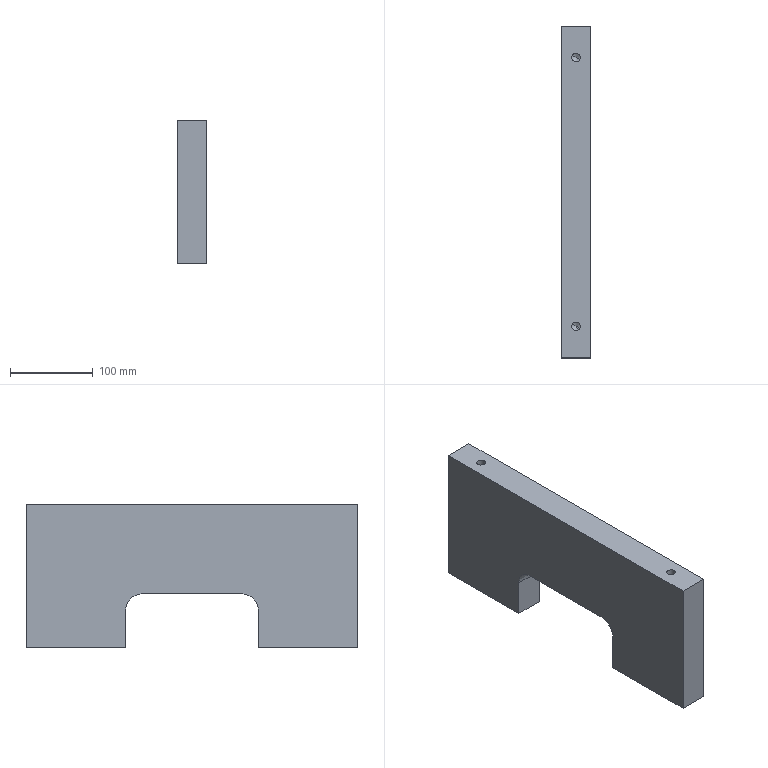Part | CATIA | 1 solid | 28 faces | box 35 x 400 x 173 mm | volume 2052248 mm3 | plane 10 | cylinder 10 | cone 8 | commonest cylinder face diameters 10.2 x8 40 x2
STEP:
#1=CARTESIAN_POINT('',(17.5,200.,-102.));
#2=VERTEX_POINT('',#1);
#3=CARTESIAN_POINT('',(17.5,200.,-275.));
#4=VERTEX_POINT('',#3);
#5=CARTESIAN_POINT('',(17.5,200.,-188.5));
#6=DIRECTION('',(0.,0.,-1.));
#7=VECTOR('',#6,1.);
#8=LINE('',#5,#7);
#9=EDGE_CURVE('',#2,#4,#8,.T.);
#10=ORIENTED_EDGE('',*,*,#9,.T.);
#11=CARTESIAN_POINT('',(-17.5,200.,-275.));
#12=VERTEX_POINT('',#11);
#13=CARTESIAN_POINT('',(0.,200.,-275.));
#14=DIRECTION('',(1.,0.,0.));
#15=VECTOR('',#14,1.);
#16=LINE('',#13,#15);
#17=EDGE_CURVE('',#4,#12,#16,.F.);
#18=ORIENTED_EDGE('',*,*,#17,.T.);
#19=CARTESIAN_POINT('',(-17.5,200.,-102.));
#20=VERTEX_POINT('',#19);
#21=CARTESIAN_POINT('',(-17.5,200.,-188.5));
#22=DIRECTION('',(0.,0.,-1.));
#23=VECTOR('',#22,1.);
#24=LINE('',#21,#23);
#25=EDGE_CURVE('',#20,#12,#24,.T.);
#26=ORIENTED_EDGE('',*,*,#25,.F.);
#27=CARTESIAN_POINT('',(0.,200.,-102.));
#28=DIRECTION('',(1.,0.,0.));
#29=VECTOR('',#28,1.);
#30=LINE('',#27,#29);
#31=EDGE_CURVE('',#20,#2,#30,.T.);
#32=ORIENTED_EDGE('',*,*,#31,.T.);
#33=EDGE_LOOP('',(#10,#18,#26,#32));
#34=FACE_OUTER_BOUND('',#33,.T.);
#35=CARTESIAN_POINT('',(-17.5,200.,0.));
#36=DIRECTION('',(0.,1.,0.));
#37=DIRECTION('',(1.,0.,0.));
#38=AXIS2_PLACEMENT_3D('',#35,#36,#37);
#39=PLANE('',#38);
#40=ADVANCED_FACE('',(#34),#39,.T.);
#41=CARTESIAN_POINT('',(-17.5,-200.,-102.));
#42=VERTEX_POINT('',#41);
#43=CARTESIAN_POINT('',(-17.5,-200.,-275.));
#44=VERTEX_POINT('',#43);
#45=CARTESIAN_POINT('',(-17.5,-200.,-188.5));
#46=DIRECTION('',(0.,0.,-1.));
#47=VECTOR('',#46,1.);
#48=LINE('',#45,#47);
#49=EDGE_CURVE('',#42,#44,#48,.T.);
#50=ORIENTED_EDGE('',*,*,#49,.T.);
#51=CARTESIAN_POINT('',(17.5,-200.,-275.));
#52=VERTEX_POINT('',#51);
#53=CARTESIAN_POINT('',(0.,-200.,-275.));
#54=DIRECTION('',(-1.,0.,0.));
#55=VECTOR('',#54,1.);
#56=LINE('',#53,#55);
#57=EDGE_CURVE('',#44,#52,#56,.F.);
#58=ORIENTED_EDGE('',*,*,#57,.T.);
#59=CARTESIAN_POINT('',(17.5,-200.,-102.));
#60=VERTEX_POINT('',#59);
#61=CARTESIAN_POINT('',(17.5,-200.,-188.5));
#62=DIRECTION('',(0.,0.,-1.));
#63=VECTOR('',#62,1.);
#64=LINE('',#61,#63);
#65=EDGE_CURVE('',#60,#52,#64,.T.);
#66=ORIENTED_EDGE('',*,*,#65,.F.);
#67=CARTESIAN_POINT('',(0.,-200.,-102.));
#68=DIRECTION('',(-1.,0.,0.));
#69=VECTOR('',#68,1.);
#70=LINE('',#67,#69);
#71=EDGE_CURVE('',#60,#42,#70,.T.);
#72=ORIENTED_EDGE('',*,*,#71,.T.);
#73=EDGE_LOOP('',(#50,#58,#66,#72));
#74=FACE_OUTER_BOUND('',#73,.T.);
#75=CARTESIAN_POINT('',(17.5,-200.,0.));
#76=DIRECTION('',(0.,-1.,0.));
#77=DIRECTION('',(-1.,0.,0.));
#78=AXIS2_PLACEMENT_3D('',#75,#76,#77);
#79=PLANE('',#78);
#80=ADVANCED_FACE('',(#74),#79,.T.);
#81=CARTESIAN_POINT('',(-17.5,80.,-275.));
#82=VERTEX_POINT('',#81);
#83=CARTESIAN_POINT('',(-17.5,80.,-230.));
#84=VERTEX_POINT('',#83);
#85=CARTESIAN_POINT('',(-17.5,80.,-252.5));
#86=DIRECTION('',(0.,0.,1.));
#87=VECTOR('',#86,1.);
#88=LINE('',#85,#87);
#89=EDGE_CURVE('',#82,#84,#88,.T.);
#90=ORIENTED_EDGE('',*,*,#89,.T.);
#91=CARTESIAN_POINT('',(-17.5,60.,-210.));
#92=VERTEX_POINT('',#91);
#93=CARTESIAN_POINT('',(-17.5,60.,-230.));
#94=DIRECTION('',(1.,0.,0.));
#95=AXIS2_PLACEMENT_3D('',#93,#94,$);
#96=CIRCLE('',#95,20.);
#97=EDGE_CURVE('',#84,#92,#96,.T.);
#98=ORIENTED_EDGE('',*,*,#97,.T.);
#99=CARTESIAN_POINT('',(-17.5,-60.,-210.));
#100=VERTEX_POINT('',#99);
#101=CARTESIAN_POINT('',(-17.5,0.,-210.));
#102=DIRECTION('',(0.,1.,0.));
#103=VECTOR('',#102,1.);
#104=LINE('',#101,#103);
#105=EDGE_CURVE('',#100,#92,#104,.T.);
#106=ORIENTED_EDGE('',*,*,#105,.F.);
#107=CARTESIAN_POINT('',(-17.5,-80.,-230.));
#108=VERTEX_POINT('',#107);
#109=CARTESIAN_POINT('',(-17.5,-60.,-230.));
#110=DIRECTION('',(1.,0.,0.));
#111=AXIS2_PLACEMENT_3D('',#109,#110,$);
#112=CIRCLE('',#111,20.);
#113=EDGE_CURVE('',#100,#108,#112,.T.);
#114=ORIENTED_EDGE('',*,*,#113,.T.);
#115=CARTESIAN_POINT('',(-17.5,-80.,-275.));
#116=VERTEX_POINT('',#115);
#117=CARTESIAN_POINT('',(-17.5,-80.,-252.5));
#118=DIRECTION('',(0.,0.,1.));
#119=VECTOR('',#118,1.);
#120=LINE('',#117,#119);
#121=EDGE_CURVE('',#116,#108,#120,.T.);
#122=ORIENTED_EDGE('',*,*,#121,.F.);
#123=CARTESIAN_POINT('',(-17.5,-140.,-275.));
#124=DIRECTION('',(0.,-1.,0.));
#125=VECTOR('',#124,1.);
#126=LINE('',#123,#125);
#127=EDGE_CURVE('',#116,#44,#126,.T.);
#128=ORIENTED_EDGE('',*,*,#127,.T.);
#129=ORIENTED_EDGE('',*,*,#49,.F.);
#130=CARTESIAN_POINT('',(-17.5,0.,-102.));
#131=DIRECTION('',(0.,-1.,0.));
#132=VECTOR('',#131,1.);
#133=LINE('',#130,#132);
#134=EDGE_CURVE('',#20,#42,#133,.T.);
#135=ORIENTED_EDGE('',*,*,#134,.F.);
#136=ORIENTED_EDGE('',*,*,#25,.T.);
#137=CARTESIAN_POINT('',(-17.5,140.,-275.));
#138=DIRECTION('',(0.,-1.,0.));
#139=VECTOR('',#138,1.);
#140=LINE('',#137,#139);
#141=EDGE_CURVE('',#12,#82,#140,.T.);
#142=ORIENTED_EDGE('',*,*,#141,.T.);
#143=EDGE_LOOP('',(#90,#98,#106,#114,#122,#128,#129,#135,#136,#142));
#144=FACE_OUTER_BOUND('',#143,.T.);
#145=CARTESIAN_POINT('',(-17.5,200.,0.));
#146=DIRECTION('',(1.,0.,0.));
#147=DIRECTION('',(0.,-1.,0.));
#148=AXIS2_PLACEMENT_3D('',#145,#146,#147);
#149=PLANE('',#148);
#150=ADVANCED_FACE('',(#144),#149,.F.);
#151=CARTESIAN_POINT('',(17.5,-80.,-275.));
#152=VERTEX_POINT('',#151);
#153=CARTESIAN_POINT('',(17.5,-80.,-230.));
#154=VERTEX_POINT('',#153);
#155=CARTESIAN_POINT('',(17.5,-80.,-252.5));
#156=DIRECTION('',(0.,0.,1.));
#157=VECTOR('',#156,1.);
#158=LINE('',#155,#157);
#159=EDGE_CURVE('',#152,#154,#158,.T.);
#160=ORIENTED_EDGE('',*,*,#159,.T.);
#161=CARTESIAN_POINT('',(17.5,-60.,-210.));
#162=VERTEX_POINT('',#161);
#163=CARTESIAN_POINT('',(17.5,-60.,-230.));
#164=DIRECTION('',(-1.,0.,0.));
#165=AXIS2_PLACEMENT_3D('',#163,#164,$);
#166=CIRCLE('',#165,20.);
#167=EDGE_CURVE('',#154,#162,#166,.T.);
#168=ORIENTED_EDGE('',*,*,#167,.T.);
#169=CARTESIAN_POINT('',(17.5,60.,-210.));
#170=VERTEX_POINT('',#169);
#171=CARTESIAN_POINT('',(17.5,0.,-210.));
#172=DIRECTION('',(0.,1.,0.));
#173=VECTOR('',#172,1.);
#174=LINE('',#171,#173);
#175=EDGE_CURVE('',#162,#170,#174,.T.);
#176=ORIENTED_EDGE('',*,*,#175,.T.);
#177=CARTESIAN_POINT('',(17.5,80.,-230.));
#178=VERTEX_POINT('',#177);
#179=CARTESIAN_POINT('',(17.5,60.,-230.));
#180=DIRECTION('',(-1.,0.,0.));
#181=AXIS2_PLACEMENT_3D('',#179,#180,$);
#182=CIRCLE('',#181,20.);
#183=EDGE_CURVE('',#170,#178,#182,.T.);
#184=ORIENTED_EDGE('',*,*,#183,.T.);
#185=CARTESIAN_POINT('',(17.5,80.,-275.));
#186=VERTEX_POINT('',#185);
#187=CARTESIAN_POINT('',(17.5,80.,-252.5));
#188=DIRECTION('',(0.,0.,1.));
#189=VECTOR('',#188,1.);
#190=LINE('',#187,#189);
#191=EDGE_CURVE('',#186,#178,#190,.T.);
#192=ORIENTED_EDGE('',*,*,#191,.F.);
#193=CARTESIAN_POINT('',(17.5,140.,-275.));
#194=DIRECTION('',(0.,1.,0.));
#195=VECTOR('',#194,1.);
#196=LINE('',#193,#195);
#197=EDGE_CURVE('',#186,#4,#196,.T.);
#198=ORIENTED_EDGE('',*,*,#197,.T.);
#199=ORIENTED_EDGE('',*,*,#9,.F.);
#200=CARTESIAN_POINT('',(17.5,0.,-102.));
#201=DIRECTION('',(0.,1.,0.));
#202=VECTOR('',#201,1.);
#203=LINE('',#200,#202);
#204=EDGE_CURVE('',#60,#2,#203,.T.);
#205=ORIENTED_EDGE('',*,*,#204,.F.);
#206=ORIENTED_EDGE('',*,*,#65,.T.);
#207=CARTESIAN_POINT('',(17.5,-140.,-275.));
#208=DIRECTION('',(0.,1.,0.));
#209=VECTOR('',#208,1.);
#210=LINE('',#207,#209);
#211=EDGE_CURVE('',#52,#152,#210,.T.);
#212=ORIENTED_EDGE('',*,*,#211,.T.);
#213=EDGE_LOOP('',(#160,#168,#176,#184,#192,#198,#199,#205,#206,#212));
#214=FACE_OUTER_BOUND('',#213,.T.);
#215=CARTESIAN_POINT('',(17.5,-200.,0.));
#216=DIRECTION('',(-1.,0.,0.));
#217=DIRECTION('',(0.,1.,0.));
#218=AXIS2_PLACEMENT_3D('',#215,#216,#217);
#219=PLANE('',#218);
#220=ADVANCED_FACE('',(#214),#219,.F.);
#221=CARTESIAN_POINT('',(0.,-80.,-230.));
#222=DIRECTION('',(1.,0.,0.));
#223=VECTOR('',#222,1.);
#224=LINE('',#221,#223);
#225=EDGE_CURVE('',#154,#108,#224,.F.);
#226=ORIENTED_EDGE('',*,*,#225,.T.);
#227=ORIENTED_EDGE('',*,*,#113,.F.);
#228=CARTESIAN_POINT('',(0.,-60.,-210.));
#229=DIRECTION('',(1.,0.,0.));
#230=VECTOR('',#229,1.);
#231=LINE('',#228,#230);
#232=EDGE_CURVE('',#162,#100,#231,.F.);
#233=ORIENTED_EDGE('',*,*,#232,.F.);
#234=ORIENTED_EDGE('',*,*,#167,.F.);
#235=EDGE_LOOP('',(#226,#227,#233,#234));
#236=FACE_OUTER_BOUND('',#235,.T.);
#237=CARTESIAN_POINT('',(0.,-60.,-230.));
#238=DIRECTION('',(1.,0.,0.));
#239=DIRECTION('',(0.,0.,1.));
#240=AXIS2_PLACEMENT_3D('',#237,#238,#239);
#241=CYLINDRICAL_SURFACE('',#240,20.);
#242=ADVANCED_FACE('',(#236),#241,.F.);
#243=ORIENTED_EDGE('',*,*,#175,.F.);
#244=ORIENTED_EDGE('',*,*,#232,.T.);
#245=ORIENTED_EDGE('',*,*,#105,.T.);
#246=CARTESIAN_POINT('',(0.,60.,-210.));
#247=DIRECTION('',(-1.,0.,0.));
#248=VECTOR('',#247,1.);
#249=LINE('',#246,#248);
#250=EDGE_CURVE('',#92,#170,#249,.F.);
#251=ORIENTED_EDGE('',*,*,#250,.T.);
#252=EDGE_LOOP('',(#243,#244,#245,#251));
#253=FACE_OUTER_BOUND('',#252,.T.);
#254=CARTESIAN_POINT('',(0.,0.,-210.));
#255=DIRECTION('',(0.,0.,-1.));
#256=DIRECTION('',(1.,0.,0.));
#257=AXIS2_PLACEMENT_3D('',#254,#255,#256);
#258=PLANE('',#257);
#259=ADVANCED_FACE('',(#253),#258,.T.);
#260=CARTESIAN_POINT('',(0.,-80.,-275.));
#261=DIRECTION('',(1.,0.,0.));
#262=VECTOR('',#261,1.);
#263=LINE('',#260,#262);
#264=EDGE_CURVE('',#152,#116,#263,.F.);
#265=ORIENTED_EDGE('',*,*,#264,.T.);
#266=ORIENTED_EDGE('',*,*,#121,.T.);
#267=ORIENTED_EDGE('',*,*,#225,.F.);
#268=ORIENTED_EDGE('',*,*,#159,.F.);
#269=EDGE_LOOP('',(#265,#266,#267,#268));
#270=FACE_OUTER_BOUND('',#269,.T.);
#271=CARTESIAN_POINT('',(-25.,-80.,-275.));
#272=DIRECTION('',(0.,-1.,0.));
#273=DIRECTION('',(1.,0.,0.));
#274=AXIS2_PLACEMENT_3D('',#271,#272,#273);
#275=PLANE('',#274);
#276=ADVANCED_FACE('',(#270),#275,.F.);
#277=CARTESIAN_POINT('',(0.,80.,-230.));
#278=DIRECTION('',(-1.,0.,0.));
#279=VECTOR('',#278,1.);
#280=LINE('',#277,#279);
#281=EDGE_CURVE('',#84,#178,#280,.F.);
#282=ORIENTED_EDGE('',*,*,#281,.T.);
#283=ORIENTED_EDGE('',*,*,#183,.F.);
#284=ORIENTED_EDGE('',*,*,#250,.F.);
#285=ORIENTED_EDGE('',*,*,#97,.F.);
#286=EDGE_LOOP('',(#282,#283,#284,#285));
#287=FACE_OUTER_BOUND('',#286,.T.);
#288=CARTESIAN_POINT('',(0.,60.,-230.));
#289=DIRECTION('',(-1.,0.,0.));
#290=DIRECTION('',(0.,0.,1.));
#291=AXIS2_PLACEMENT_3D('',#288,#289,#290);
#292=CYLINDRICAL_SURFACE('',#291,20.);
#293=ADVANCED_FACE('',(#287),#292,.F.);
#294=CARTESIAN_POINT('',(0.,80.,-275.));
#295=DIRECTION('',(-1.,0.,0.));
#296=VECTOR('',#295,1.);
#297=LINE('',#294,#296);
#298=EDGE_CURVE('',#82,#186,#297,.F.);
#299=ORIENTED_EDGE('',*,*,#298,.T.);
#300=ORIENTED_EDGE('',*,*,#191,.T.);
#301=ORIENTED_EDGE('',*,*,#281,.F.);
#302=ORIENTED_EDGE('',*,*,#89,.F.);
#303=EDGE_LOOP('',(#299,#300,#301,#302));
#304=FACE_OUTER_BOUND('',#303,.T.);
#305=CARTESIAN_POINT('',(25.,80.,-275.));
#306=DIRECTION('',(0.,1.,0.));
#307=DIRECTION('',(-1.,0.,0.));
#308=AXIS2_PLACEMENT_3D('',#305,#306,#307);
#309=PLANE('',#308);
#310=ADVANCED_FACE('',(#304),#309,.F.);
#311=ORIENTED_EDGE('',*,*,#298,.F.);
#312=ORIENTED_EDGE('',*,*,#141,.F.);
#313=ORIENTED_EDGE('',*,*,#17,.F.);
#314=ORIENTED_EDGE('',*,*,#197,.F.);
#315=EDGE_LOOP('',(#311,#312,#313,#314));
#316=FACE_OUTER_BOUND('',#315,.T.);
#317=CARTESIAN_POINT('',(4.476,177.445,-275.));
#318=VERTEX_POINT('',#317);
#319=CARTESIAN_POINT('',(-4.476,172.555,-275.));
#320=VERTEX_POINT('',#319);
#321=CARTESIAN_POINT('',(0.,175.,-275.));
#322=DIRECTION('',(0.,0.,1.));
#323=AXIS2_PLACEMENT_3D('',#321,#322,$);
#324=CIRCLE('',#323,5.1);
#325=EDGE_CURVE('',#318,#320,#324,.T.);
#326=ORIENTED_EDGE('',*,*,#325,.T.);
#327=CARTESIAN_POINT('',(0.,175.,-275.));
#328=DIRECTION('',(0.,0.,1.));
#329=AXIS2_PLACEMENT_3D('',#327,#328,$);
#330=CIRCLE('',#329,5.1);
#331=EDGE_CURVE('',#320,#318,#330,.T.);
#332=ORIENTED_EDGE('',*,*,#331,.T.);
#333=EDGE_LOOP('',(#326,#332));
#334=FACE_BOUND('',#333,.T.);
#335=CARTESIAN_POINT('',(0.,0.,-275.));
#336=DIRECTION('',(0.,0.,1.));
#337=DIRECTION('',(1.,0.,0.));
#338=AXIS2_PLACEMENT_3D('',#335,#336,#337);
#339=PLANE('',#338);
#340=ADVANCED_FACE('',(#316,#334),#339,.F.);
#341=ORIENTED_EDGE('',*,*,#264,.F.);
#342=ORIENTED_EDGE('',*,*,#211,.F.);
#343=ORIENTED_EDGE('',*,*,#57,.F.);
#344=ORIENTED_EDGE('',*,*,#127,.F.);
#345=EDGE_LOOP('',(#341,#342,#343,#344));
#346=FACE_OUTER_BOUND('',#345,.T.);
#347=CARTESIAN_POINT('',(4.476,-167.555,-275.));
#348=VERTEX_POINT('',#347);
#349=CARTESIAN_POINT('',(-4.476,-172.445,-275.));
#350=VERTEX_POINT('',#349);
#351=CARTESIAN_POINT('',(0.,-170.,-275.));
#352=DIRECTION('',(0.,0.,1.));
#353=AXIS2_PLACEMENT_3D('',#351,#352,$);
#354=CIRCLE('',#353,5.1);
#355=EDGE_CURVE('',#348,#350,#354,.T.);
#356=ORIENTED_EDGE('',*,*,#355,.T.);
#357=CARTESIAN_POINT('',(0.,-170.,-275.));
#358=DIRECTION('',(0.,0.,1.));
#359=AXIS2_PLACEMENT_3D('',#357,#358,$);
#360=CIRCLE('',#359,5.1);
#361=EDGE_CURVE('',#350,#348,#360,.T.);
#362=ORIENTED_EDGE('',*,*,#361,.T.);
#363=EDGE_LOOP('',(#356,#362));
#364=FACE_BOUND('',#363,.T.);
#365=ADVANCED_FACE('',(#346,#364),#339,.F.);
#366=ORIENTED_EDGE('',*,*,#31,.F.);
#367=ORIENTED_EDGE('',*,*,#134,.T.);
#368=ORIENTED_EDGE('',*,*,#71,.F.);
#369=ORIENTED_EDGE('',*,*,#204,.T.);
#370=EDGE_LOOP('',(#366,#367,#368,#369));
#371=FACE_OUTER_BOUND('',#370,.T.);
#372=CARTESIAN_POINT('',(4.476,-164.445,-102.));
#373=VERTEX_POINT('',#372);
#374=CARTESIAN_POINT('',(-4.476,-159.555,-102.));
#375=VERTEX_POINT('',#374);
#376=CARTESIAN_POINT('',(0.,-162.,-102.));
#377=DIRECTION('',(0.,0.,1.));
#378=AXIS2_PLACEMENT_3D('',#376,#377,$);
#379=CIRCLE('',#378,5.1);
#380=EDGE_CURVE('',#373,#375,#379,.T.);
#381=ORIENTED_EDGE('',*,*,#380,.F.);
#382=CARTESIAN_POINT('',(0.,-162.,-102.));
#383=DIRECTION('',(0.,0.,1.));
#384=AXIS2_PLACEMENT_3D('',#382,#383,$);
#385=CIRCLE('',#384,5.1);
#386=EDGE_CURVE('',#375,#373,#385,.T.);
#387=ORIENTED_EDGE('',*,*,#386,.F.);
#388=EDGE_LOOP('',(#381,#387));
#389=FACE_BOUND('',#388,.T.);
#390=CARTESIAN_POINT('',(4.476,159.555,-102.));
#391=VERTEX_POINT('',#390);
#392=CARTESIAN_POINT('',(-4.476,164.445,-102.));
#393=VERTEX_POINT('',#392);
#394=CARTESIAN_POINT('',(0.,162.,-102.));
#395=DIRECTION('',(0.,0.,1.));
#396=AXIS2_PLACEMENT_3D('',#394,#395,$);
#397=CIRCLE('',#396,5.1);
#398=EDGE_CURVE('',#391,#393,#397,.T.);
#399=ORIENTED_EDGE('',*,*,#398,.F.);
#400=CARTESIAN_POINT('',(0.,162.,-102.));
#401=DIRECTION('',(0.,0.,1.));
#402=AXIS2_PLACEMENT_3D('',#400,#401,$);
#403=CIRCLE('',#402,5.1);
#404=EDGE_CURVE('',#393,#391,#403,.T.);
#405=ORIENTED_EDGE('',*,*,#404,.F.);
#406=EDGE_LOOP('',(#399,#405));
#407=FACE_BOUND('',#406,.T.);
#408=CARTESIAN_POINT('',(0.,0.,-102.));
#409=DIRECTION('',(0.,0.,1.));
#410=DIRECTION('',(1.,0.,0.));
#411=AXIS2_PLACEMENT_3D('',#408,#409,#410);
#412=PLANE('',#411);
#413=ADVANCED_FACE('',(#371,#389,#407),#412,.T.);
#414=CARTESIAN_POINT('',(0.,162.,-139.944));
#415=VERTEX_POINT('',#414);
#416=CARTESIAN_POINT('',(-4.476,164.445,-137.));
#417=VERTEX_POINT('',#416);
#418=CARTESIAN_POINT('',(-2.238,163.223,-138.472));
#419=DIRECTION('',(-0.76,0.4152,0.5));
#420=VECTOR('',#419,1.);
#421=LINE('',#418,#420);
#422=EDGE_CURVE('',#415,#417,#421,.T.);
#423=ORIENTED_EDGE('',*,*,#422,.T.);
#424=CARTESIAN_POINT('',(4.476,159.555,-137.));
#425=VERTEX_POINT('',#424);
#426=CARTESIAN_POINT('',(0.,162.,-137.));
#427=DIRECTION('',(0.,0.,1.));
#428=AXIS2_PLACEMENT_3D('',#426,#427,$);
#429=CIRCLE('',#428,5.1);
#430=EDGE_CURVE('',#425,#417,#429,.F.);
#431=ORIENTED_EDGE('',*,*,#430,.F.);
#432=CARTESIAN_POINT('',(2.238,160.777,-138.472));
#433=DIRECTION('',(0.76,-0.4152,0.5));
#434=VECTOR('',#433,1.);
#435=LINE('',#432,#434);
#436=EDGE_CURVE('',#415,#425,#435,.T.);
#437=ORIENTED_EDGE('',*,*,#436,.F.);
#438=EDGE_LOOP('',(#423,#431,#437));
#439=FACE_OUTER_BOUND('',#438,.T.);
#440=CARTESIAN_POINT('',(0.,162.,-139.944));
#441=DIRECTION('',(0.,0.,1.));
#442=DIRECTION('',(0.8776,-0.4794,0.));
#443=AXIS2_PLACEMENT_3D('',#440,#441,#442);
#444=CONICAL_SURFACE('',#443,0.,1.047);
#445=ADVANCED_FACE('',(#439),#444,.F.);
#446=ORIENTED_EDGE('',*,*,#436,.T.);
#447=CARTESIAN_POINT('',(0.,162.,-137.));
#448=DIRECTION('',(0.,0.,1.));
#449=AXIS2_PLACEMENT_3D('',#447,#448,$);
#450=CIRCLE('',#449,5.1);
#451=EDGE_CURVE('',#417,#425,#450,.F.);
#452=ORIENTED_EDGE('',*,*,#451,.F.);
#453=ORIENTED_EDGE('',*,*,#422,.F.);
#454=EDGE_LOOP('',(#446,#452,#453));
#455=FACE_OUTER_BOUND('',#454,.T.);
#456=ADVANCED_FACE('',(#455),#444,.F.);
#457=ORIENTED_EDGE('',*,*,#404,.T.);
#458=CARTESIAN_POINT('',(4.476,159.555,-119.3));
#459=DIRECTION('',(0.,0.,-1.));
#460=VECTOR('',#459,1.);
#461=LINE('',#458,#460);
#462=EDGE_CURVE('',#425,#391,#461,.F.);
#463=ORIENTED_EDGE('',*,*,#462,.F.);
#464=ORIENTED_EDGE('',*,*,#430,.T.);
#465=CARTESIAN_POINT('',(-4.476,164.445,-119.3));
#466=DIRECTION('',(0.,0.,-1.));
#467=VECTOR('',#466,1.);
#468=LINE('',#465,#467);
#469=EDGE_CURVE('',#417,#393,#468,.F.);
#470=ORIENTED_EDGE('',*,*,#469,.T.);
#471=EDGE_LOOP('',(#457,#463,#464,#470));
#472=FACE_OUTER_BOUND('',#471,.T.);
#473=CARTESIAN_POINT('',(0.,162.,-102.1));
#474=DIRECTION('',(0.,0.,-1.));
#475=DIRECTION('',(0.8776,-0.4794,0.));
#476=AXIS2_PLACEMENT_3D('',#473,#474,#475);
#477=CYLINDRICAL_SURFACE('',#476,5.1);
#478=ADVANCED_FACE('',(#472),#477,.F.);
#479=ORIENTED_EDGE('',*,*,#398,.T.);
#480=ORIENTED_EDGE('',*,*,#469,.F.);
#481=ORIENTED_EDGE('',*,*,#451,.T.);
#482=ORIENTED_EDGE('',*,*,#462,.T.);
#483=EDGE_LOOP('',(#479,#480,#481,#482));
#484=FACE_OUTER_BOUND('',#483,.T.);
#485=ADVANCED_FACE('',(#484),#477,.F.);
#486=CARTESIAN_POINT('',(0.,-162.,-139.944));
#487=VERTEX_POINT('',#486);
#488=CARTESIAN_POINT('',(-4.476,-159.555,-137.));
#489=VERTEX_POINT('',#488);
#490=CARTESIAN_POINT('',(-2.238,-160.777,-138.472));
#491=DIRECTION('',(-0.76,0.4152,0.5));
#492=VECTOR('',#491,1.);
#493=LINE('',#490,#492);
#494=EDGE_CURVE('',#487,#489,#493,.T.);
#495=ORIENTED_EDGE('',*,*,#494,.T.);
#496=CARTESIAN_POINT('',(4.476,-164.445,-137.));
#497=VERTEX_POINT('',#496);
#498=CARTESIAN_POINT('',(0.,-162.,-137.));
#499=DIRECTION('',(0.,0.,1.));
#500=AXIS2_PLACEMENT_3D('',#498,#499,$);
#501=CIRCLE('',#500,5.1);
#502=EDGE_CURVE('',#497,#489,#501,.F.);
#503=ORIENTED_EDGE('',*,*,#502,.F.);
#504=CARTESIAN_POINT('',(2.238,-163.223,-138.472));
#505=DIRECTION('',(0.76,-0.4152,0.5));
#506=VECTOR('',#505,1.);
#507=LINE('',#504,#506);
#508=EDGE_CURVE('',#487,#497,#507,.T.);
#509=ORIENTED_EDGE('',*,*,#508,.F.);
#510=EDGE_LOOP('',(#495,#503,#509));
#511=FACE_OUTER_BOUND('',#510,.T.);
#512=CARTESIAN_POINT('',(0.,-162.,-139.944));
#513=DIRECTION('',(0.,0.,1.));
#514=DIRECTION('',(0.8776,-0.4794,0.));
#515=AXIS2_PLACEMENT_3D('',#512,#513,#514);
#516=CONICAL_SURFACE('',#515,0.,1.047);
#517=ADVANCED_FACE('',(#511),#516,.F.);
#518=ORIENTED_EDGE('',*,*,#508,.T.);
#519=CARTESIAN_POINT('',(0.,-162.,-137.));
#520=DIRECTION('',(0.,0.,1.));
#521=AXIS2_PLACEMENT_3D('',#519,#520,$);
#522=CIRCLE('',#521,5.1);
#523=EDGE_CURVE('',#489,#497,#522,.F.);
#524=ORIENTED_EDGE('',*,*,#523,.F.);
#525=ORIENTED_EDGE('',*,*,#494,.F.);
#526=EDGE_LOOP('',(#518,#524,#525));
#527=FACE_OUTER_BOUND('',#526,.T.);
#528=ADVANCED_FACE('',(#527),#516,.F.);
#529=ORIENTED_EDGE('',*,*,#386,.T.);
#530=CARTESIAN_POINT('',(4.476,-164.445,-119.3));
#531=DIRECTION('',(0.,0.,-1.));
#532=VECTOR('',#531,1.);
#533=LINE('',#530,#532);
#534=EDGE_CURVE('',#497,#373,#533,.F.);
#535=ORIENTED_EDGE('',*,*,#534,.F.);
#536=ORIENTED_EDGE('',*,*,#502,.T.);
#537=CARTESIAN_POINT('',(-4.476,-159.555,-119.3));
#538=DIRECTION('',(0.,0.,-1.));
#539=VECTOR('',#538,1.);
#540=LINE('',#537,#539);
#541=EDGE_CURVE('',#489,#375,#540,.F.);
#542=ORIENTED_EDGE('',*,*,#541,.T.);
#543=EDGE_LOOP('',(#529,#535,#536,#542));
#544=FACE_OUTER_BOUND('',#543,.T.);
#545=CARTESIAN_POINT('',(0.,-162.,-102.1));
#546=DIRECTION('',(0.,0.,-1.));
#547=DIRECTION('',(0.8776,-0.4794,0.));
#548=AXIS2_PLACEMENT_3D('',#545,#546,#547);
#549=CYLINDRICAL_SURFACE('',#548,5.1);
#550=ADVANCED_FACE('',(#544),#549,.F.);
#551=ORIENTED_EDGE('',*,*,#380,.T.);
#552=ORIENTED_EDGE('',*,*,#541,.F.);
#553=ORIENTED_EDGE('',*,*,#523,.T.);
#554=ORIENTED_EDGE('',*,*,#534,.T.);
#555=EDGE_LOOP('',(#551,#552,#553,#554));
#556=FACE_OUTER_BOUND('',#555,.T.);
#557=ADVANCED_FACE('',(#556),#549,.F.);
#558=CARTESIAN_POINT('',(0.,-170.,-237.056));
#559=VERTEX_POINT('',#558);
#560=CARTESIAN_POINT('',(-4.476,-172.445,-240.));
#561=VERTEX_POINT('',#560);
#562=CARTESIAN_POINT('',(-2.238,-171.223,-238.528));
#563=DIRECTION('',(-0.76,-0.4152,-0.5));
#564=VECTOR('',#563,1.);
#565=LINE('',#562,#564);
#566=EDGE_CURVE('',#559,#561,#565,.T.);
#567=ORIENTED_EDGE('',*,*,#566,.T.);
#568=CARTESIAN_POINT('',(4.476,-167.555,-240.));
#569=VERTEX_POINT('',#568);
#570=CARTESIAN_POINT('',(0.,-170.,-240.));
#571=DIRECTION('',(0.,0.,-1.));
#572=AXIS2_PLACEMENT_3D('',#570,#571,$);
#573=CIRCLE('',#572,5.1);
#574=EDGE_CURVE('',#569,#561,#573,.F.);
#575=ORIENTED_EDGE('',*,*,#574,.F.);
#576=CARTESIAN_POINT('',(2.238,-168.777,-238.528));
#577=DIRECTION('',(0.76,0.4152,-0.5));
#578=VECTOR('',#577,1.);
#579=LINE('',#576,#578);
#580=EDGE_CURVE('',#559,#569,#579,.T.);
#581=ORIENTED_EDGE('',*,*,#580,.F.);
#582=EDGE_LOOP('',(#567,#575,#581));
#583=FACE_OUTER_BOUND('',#582,.T.);
#584=CARTESIAN_POINT('',(0.,-170.,-237.056));
#585=DIRECTION('',(0.,0.,-1.));
#586=DIRECTION('',(0.8776,0.4794,0.));
#587=AXIS2_PLACEMENT_3D('',#584,#585,#586);
#588=CONICAL_SURFACE('',#587,0.,1.047);
#589=ADVANCED_FACE('',(#583),#588,.F.);
#590=ORIENTED_EDGE('',*,*,#580,.T.);
#591=CARTESIAN_POINT('',(0.,-170.,-240.));
#592=DIRECTION('',(0.,0.,-1.));
#593=AXIS2_PLACEMENT_3D('',#591,#592,$);
#594=CIRCLE('',#593,5.1);
#595=EDGE_CURVE('',#561,#569,#594,.F.);
#596=ORIENTED_EDGE('',*,*,#595,.F.);
#597=ORIENTED_EDGE('',*,*,#566,.F.);
#598=EDGE_LOOP('',(#590,#596,#597));
#599=FACE_OUTER_BOUND('',#598,.T.);
#600=ADVANCED_FACE('',(#599),#588,.F.);
#601=ORIENTED_EDGE('',*,*,#355,.F.);
#602=CARTESIAN_POINT('',(4.476,-167.555,-257.7));
#603=DIRECTION('',(0.,0.,1.));
#604=VECTOR('',#603,1.);
#605=LINE('',#602,#604);
#606=EDGE_CURVE('',#569,#348,#605,.F.);
#607=ORIENTED_EDGE('',*,*,#606,.F.);
#608=ORIENTED_EDGE('',*,*,#574,.T.);
#609=CARTESIAN_POINT('',(-4.476,-172.445,-257.7));
#610=DIRECTION('',(0.,0.,1.));
#611=VECTOR('',#610,1.);
#612=LINE('',#609,#611);
#613=EDGE_CURVE('',#561,#350,#612,.F.);
#614=ORIENTED_EDGE('',*,*,#613,.T.);
#615=EDGE_LOOP('',(#601,#607,#608,#614));
#616=FACE_OUTER_BOUND('',#615,.T.);
#617=CARTESIAN_POINT('',(0.,-170.,-274.9));
#618=DIRECTION('',(0.,0.,1.));
#619=DIRECTION('',(0.8776,0.4794,0.));
#620=AXIS2_PLACEMENT_3D('',#617,#618,#619);
#621=CYLINDRICAL_SURFACE('',#620,5.1);
#622=ADVANCED_FACE('',(#616),#621,.F.);
#623=ORIENTED_EDGE('',*,*,#361,.F.);
#624=ORIENTED_EDGE('',*,*,#613,.F.);
#625=ORIENTED_EDGE('',*,*,#595,.T.);
#626=ORIENTED_EDGE('',*,*,#606,.T.);
#627=EDGE_LOOP('',(#623,#624,#625,#626));
#628=FACE_OUTER_BOUND('',#627,.T.);
#629=ADVANCED_FACE('',(#628),#621,.F.);
#630=CARTESIAN_POINT('',(0.,175.,-237.056));
#631=VERTEX_POINT('',#630);
#632=CARTESIAN_POINT('',(-4.476,172.555,-240.));
#633=VERTEX_POINT('',#632);
#634=CARTESIAN_POINT('',(-2.238,173.777,-238.528));
#635=DIRECTION('',(-0.76,-0.4152,-0.5));
#636=VECTOR('',#635,1.);
#637=LINE('',#634,#636);
#638=EDGE_CURVE('',#631,#633,#637,.T.);
#639=ORIENTED_EDGE('',*,*,#638,.T.);
#640=CARTESIAN_POINT('',(4.476,177.445,-240.));
#641=VERTEX_POINT('',#640);
#642=CARTESIAN_POINT('',(0.,175.,-240.));
#643=DIRECTION('',(0.,0.,-1.));
#644=AXIS2_PLACEMENT_3D('',#642,#643,$);
#645=CIRCLE('',#644,5.1);
#646=EDGE_CURVE('',#641,#633,#645,.F.);
#647=ORIENTED_EDGE('',*,*,#646,.F.);
#648=CARTESIAN_POINT('',(2.238,176.223,-238.528));
#649=DIRECTION('',(0.76,0.4152,-0.5));
#650=VECTOR('',#649,1.);
#651=LINE('',#648,#650);
#652=EDGE_CURVE('',#631,#641,#651,.T.);
#653=ORIENTED_EDGE('',*,*,#652,.F.);
#654=EDGE_LOOP('',(#639,#647,#653));
#655=FACE_OUTER_BOUND('',#654,.T.);
#656=CARTESIAN_POINT('',(0.,175.,-237.056));
#657=DIRECTION('',(0.,0.,-1.));
#658=DIRECTION('',(0.8776,0.4794,0.));
#659=AXIS2_PLACEMENT_3D('',#656,#657,#658);
#660=CONICAL_SURFACE('',#659,0.,1.047);
#661=ADVANCED_FACE('',(#655),#660,.F.);
#662=ORIENTED_EDGE('',*,*,#652,.T.);
#663=CARTESIAN_POINT('',(0.,175.,-240.));
#664=DIRECTION('',(0.,0.,-1.));
#665=AXIS2_PLACEMENT_3D('',#663,#664,$);
#666=CIRCLE('',#665,5.1);
#667=EDGE_CURVE('',#633,#641,#666,.F.);
#668=ORIENTED_EDGE('',*,*,#667,.F.);
#669=ORIENTED_EDGE('',*,*,#638,.F.);
#670=EDGE_LOOP('',(#662,#668,#669));
#671=FACE_OUTER_BOUND('',#670,.T.);
#672=ADVANCED_FACE('',(#671),#660,.F.);
#673=ORIENTED_EDGE('',*,*,#325,.F.);
#674=CARTESIAN_POINT('',(4.476,177.445,-257.7));
#675=DIRECTION('',(0.,0.,1.));
#676=VECTOR('',#675,1.);
#677=LINE('',#674,#676);
#678=EDGE_CURVE('',#641,#318,#677,.F.);
#679=ORIENTED_EDGE('',*,*,#678,.F.);
#680=ORIENTED_EDGE('',*,*,#646,.T.);
#681=CARTESIAN_POINT('',(-4.476,172.555,-257.7));
#682=DIRECTION('',(0.,0.,1.));
#683=VECTOR('',#682,1.);
#684=LINE('',#681,#683);
#685=EDGE_CURVE('',#633,#320,#684,.F.);
#686=ORIENTED_EDGE('',*,*,#685,.T.);
#687=EDGE_LOOP('',(#673,#679,#680,#686));
#688=FACE_OUTER_BOUND('',#687,.T.);
#689=CARTESIAN_POINT('',(0.,175.,-274.9));
#690=DIRECTION('',(0.,0.,1.));
#691=DIRECTION('',(0.8776,0.4794,0.));
#692=AXIS2_PLACEMENT_3D('',#689,#690,#691);
#693=CYLINDRICAL_SURFACE('',#692,5.1);
#694=ADVANCED_FACE('',(#688),#693,.F.);
#695=ORIENTED_EDGE('',*,*,#331,.F.);
#696=ORIENTED_EDGE('',*,*,#685,.F.);
#697=ORIENTED_EDGE('',*,*,#667,.T.);
#698=ORIENTED_EDGE('',*,*,#678,.T.);
#699=EDGE_LOOP('',(#695,#696,#697,#698));
#700=FACE_OUTER_BOUND('',#699,.T.);
#701=ADVANCED_FACE('',(#700),#693,.F.);
#702=CLOSED_SHELL('',(#40,#80,#150,#220,#242,#259,#276,#293,#310,#340,#365,#413,#445,#456,#478,#485,#517,#528,#550,#557,#589,#600,#622,#629,#661,#672,#694,#701));
#703=MANIFOLD_SOLID_BREP('',#702);
#704=(LENGTH_UNIT()NAMED_UNIT(*)SI_UNIT(.MILLI.,.METRE.));
#705=UNCERTAINTY_MEASURE_WITH_UNIT(LENGTH_MEASURE(0.005),#704,'','');
#706=(NAMED_UNIT(*)PLANE_ANGLE_UNIT()SI_UNIT($,.RADIAN.));
#707=(NAMED_UNIT(*)SI_UNIT($,.STERADIAN.)SOLID_ANGLE_UNIT());
#708=(GEOMETRIC_REPRESENTATION_CONTEXT(3)GLOBAL_UNCERTAINTY_ASSIGNED_CONTEXT((#705))GLOBAL_UNIT_ASSIGNED_CONTEXT((#704,#706,#707))REPRESENTATION_CONTEXT('',''));
#709=ADVANCED_BREP_SHAPE_REPRESENTATION('',(#703),#708);